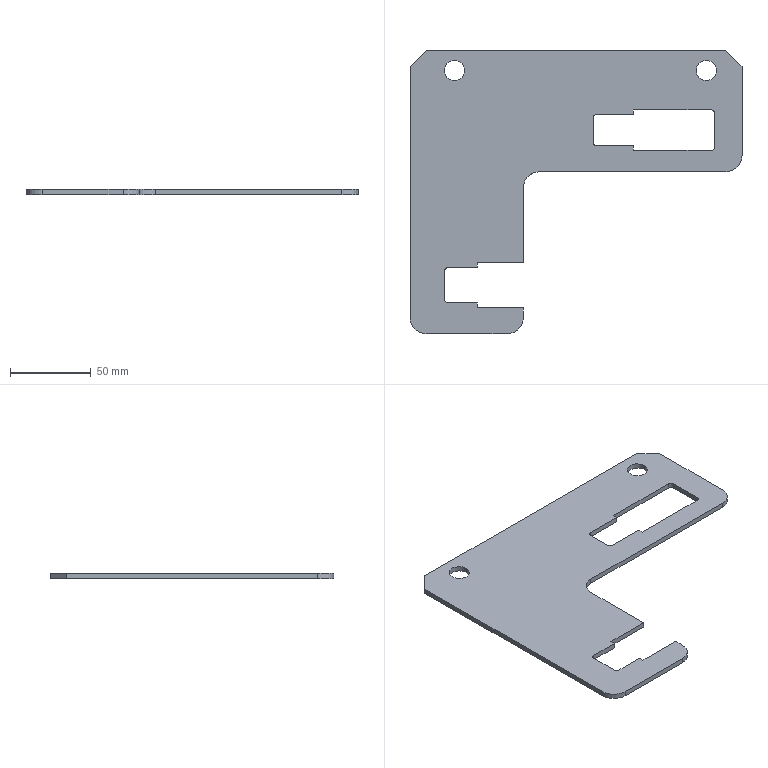Part | SolidWorks | features FlatPattern 1, SMBaseFlange 1, SheetMetal 1 | 1 solid | 40 faces | box 205 x 175 x 3.2 mm | volume 60892 mm3 | plane 26 | cylinder 14 | commonest cylinder face diameters 4 x6 12.5 x4 20 x4
STEP:
#1=CARTESIAN_POINT('',(21.25,-130.495,3.2));
#2=VERTEX_POINT('',#1);
#3=CARTESIAN_POINT('',(33.75,-130.495,3.2));
#4=VERTEX_POINT('',#3);
#5=CARTESIAN_POINT('',(27.5,-130.495,3.2));
#6=DIRECTION('',(0.,0.,1.));
#7=DIRECTION('',(1.,0.,0.));
#8=AXIS2_PLACEMENT_3D('',#5,#6,#7);
#9=CIRCLE('',#8,6.25);
#10=EDGE_CURVE('',#2,#4,#9,.T.);
#11=ORIENTED_EDGE('',*,*,#10,.T.);
#12=CARTESIAN_POINT('',(33.75,-130.495,0.));
#13=VERTEX_POINT('',#12);
#14=CARTESIAN_POINT('',(33.75,-130.495,3.2));
#15=DIRECTION('',(0.,0.,-1.));
#16=VECTOR('',#15,1000.);
#17=LINE('',#14,#16);
#18=EDGE_CURVE('',#4,#13,#17,.T.);
#19=ORIENTED_EDGE('',*,*,#18,.T.);
#20=CARTESIAN_POINT('',(21.25,-130.495,0.));
#21=VERTEX_POINT('',#20);
#22=CARTESIAN_POINT('',(27.5,-130.495,0.));
#23=DIRECTION('',(0.,0.,1.));
#24=DIRECTION('',(1.,0.,0.));
#25=AXIS2_PLACEMENT_3D('',#22,#23,#24);
#26=CIRCLE('',#25,6.25);
#27=EDGE_CURVE('',#21,#13,#26,.T.);
#28=ORIENTED_EDGE('',*,*,#27,.F.);
#29=CARTESIAN_POINT('',(21.25,-130.495,3.2));
#30=DIRECTION('',(0.,0.,-1.));
#31=VECTOR('',#30,1000.);
#32=LINE('',#29,#31);
#33=EDGE_CURVE('',#2,#21,#32,.T.);
#34=ORIENTED_EDGE('',*,*,#33,.F.);
#35=EDGE_LOOP('',(#11,#19,#28,#34));
#36=FACE_OUTER_BOUND('',#35,.T.);
#37=CARTESIAN_POINT('',(27.5,-130.495,3.2));
#38=DIRECTION('',(0.,0.,-1.));
#39=DIRECTION('',(-1.,0.,0.));
#40=AXIS2_PLACEMENT_3D('',#37,#38,#39);
#41=CYLINDRICAL_SURFACE('',#40,6.25);
#42=ADVANCED_FACE('',(#36),#41,.F.);
#43=CARTESIAN_POINT('',(176.75,-130.495,3.2));
#44=VERTEX_POINT('',#43);
#45=CARTESIAN_POINT('',(189.25,-130.495,3.2));
#46=VERTEX_POINT('',#45);
#47=CARTESIAN_POINT('',(183.,-130.495,3.2));
#48=DIRECTION('',(0.,0.,1.));
#49=DIRECTION('',(1.,0.,0.));
#50=AXIS2_PLACEMENT_3D('',#47,#48,#49);
#51=CIRCLE('',#50,6.25);
#52=EDGE_CURVE('',#44,#46,#51,.T.);
#53=ORIENTED_EDGE('',*,*,#52,.T.);
#54=CARTESIAN_POINT('',(189.25,-130.495,0.));
#55=VERTEX_POINT('',#54);
#56=CARTESIAN_POINT('',(189.25,-130.495,3.2));
#57=DIRECTION('',(0.,0.,-1.));
#58=VECTOR('',#57,1000.);
#59=LINE('',#56,#58);
#60=EDGE_CURVE('',#46,#55,#59,.T.);
#61=ORIENTED_EDGE('',*,*,#60,.T.);
#62=CARTESIAN_POINT('',(176.75,-130.495,0.));
#63=VERTEX_POINT('',#62);
#64=CARTESIAN_POINT('',(183.,-130.495,0.));
#65=DIRECTION('',(0.,0.,1.));
#66=DIRECTION('',(1.,0.,0.));
#67=AXIS2_PLACEMENT_3D('',#64,#65,#66);
#68=CIRCLE('',#67,6.25);
#69=EDGE_CURVE('',#63,#55,#68,.T.);
#70=ORIENTED_EDGE('',*,*,#69,.F.);
#71=CARTESIAN_POINT('',(176.75,-130.495,3.2));
#72=DIRECTION('',(0.,0.,-1.));
#73=VECTOR('',#72,1000.);
#74=LINE('',#71,#73);
#75=EDGE_CURVE('',#44,#63,#74,.T.);
#76=ORIENTED_EDGE('',*,*,#75,.F.);
#77=EDGE_LOOP('',(#53,#61,#70,#76));
#78=FACE_OUTER_BOUND('',#77,.T.);
#79=CARTESIAN_POINT('',(183.,-130.495,3.2));
#80=DIRECTION('',(0.,0.,-1.));
#81=DIRECTION('',(-1.,0.,0.));
#82=AXIS2_PLACEMENT_3D('',#79,#80,#81);
#83=CYLINDRICAL_SURFACE('',#82,6.25);
#84=ADVANCED_FACE('',(#78),#83,.F.);
#85=ORIENTED_EDGE('',*,*,#52,.F.);
#86=CARTESIAN_POINT('',(183.,-130.495,3.2));
#87=DIRECTION('',(0.,0.,1.));
#88=DIRECTION('',(1.,0.,0.));
#89=AXIS2_PLACEMENT_3D('',#86,#87,#88);
#90=CIRCLE('',#89,6.25);
#91=EDGE_CURVE('',#46,#44,#90,.T.);
#92=ORIENTED_EDGE('',*,*,#91,.F.);
#93=EDGE_LOOP('',(#85,#92));
#94=FACE_BOUND('',#93,.T.);
#95=CARTESIAN_POINT('',(205.,-182.995,3.2));
#96=VERTEX_POINT('',#95);
#97=CARTESIAN_POINT('',(205.,-127.995,3.2));
#98=VERTEX_POINT('',#97);
#99=CARTESIAN_POINT('',(205.,-154.795,3.2));
#100=DIRECTION('',(0.,1.,0.));
#101=VECTOR('',#100,1000.);
#102=LINE('',#99,#101);
#103=EDGE_CURVE('',#96,#98,#102,.T.);
#104=ORIENTED_EDGE('',*,*,#103,.T.);
#105=CARTESIAN_POINT('',(195.,-117.995,3.2));
#106=VERTEX_POINT('',#105);
#107=CARTESIAN_POINT('',(205.,-127.995,3.2));
#108=DIRECTION('',(-0.7071,0.7071,0.));
#109=VECTOR('',#108,1000.);
#110=LINE('',#107,#109);
#111=EDGE_CURVE('',#98,#106,#110,.T.);
#112=ORIENTED_EDGE('',*,*,#111,.T.);
#113=CARTESIAN_POINT('',(10.,-117.995,3.2));
#114=VERTEX_POINT('',#113);
#115=CARTESIAN_POINT('',(195.,-117.995,3.2));
#116=DIRECTION('',(-1.,0.,0.));
#117=VECTOR('',#116,1000.);
#118=LINE('',#115,#117);
#119=EDGE_CURVE('',#106,#114,#118,.T.);
#120=ORIENTED_EDGE('',*,*,#119,.T.);
#121=CARTESIAN_POINT('',(0.,-127.995,3.2));
#122=VERTEX_POINT('',#121);
#123=CARTESIAN_POINT('',(10.,-117.995,3.2));
#124=DIRECTION('',(-0.7071,-0.7071,0.));
#125=VECTOR('',#124,1000.);
#126=LINE('',#123,#125);
#127=EDGE_CURVE('',#114,#122,#126,.T.);
#128=ORIENTED_EDGE('',*,*,#127,.T.);
#129=CARTESIAN_POINT('',(0.,-282.995,3.2));
#130=VERTEX_POINT('',#129);
#131=CARTESIAN_POINT('',(0.,-127.995,3.2));
#132=DIRECTION('',(0.,-1.,0.));
#133=VECTOR('',#132,1000.);
#134=LINE('',#131,#133);
#135=EDGE_CURVE('',#122,#130,#134,.T.);
#136=ORIENTED_EDGE('',*,*,#135,.T.);
#137=CARTESIAN_POINT('',(10.,-292.995,3.2));
#138=VERTEX_POINT('',#137);
#139=CARTESIAN_POINT('',(10.,-282.995,3.2));
#140=DIRECTION('',(0.,0.,1.));
#141=DIRECTION('',(1.,0.,0.));
#142=AXIS2_PLACEMENT_3D('',#139,#140,#141);
#143=CIRCLE('',#142,10.);
#144=EDGE_CURVE('',#130,#138,#143,.T.);
#145=ORIENTED_EDGE('',*,*,#144,.T.);
#146=CARTESIAN_POINT('',(60.,-292.995,3.2));
#147=VERTEX_POINT('',#146);
#148=CARTESIAN_POINT('',(10.,-292.995,3.2));
#149=DIRECTION('',(1.,0.,0.));
#150=VECTOR('',#149,1000.);
#151=LINE('',#148,#150);
#152=EDGE_CURVE('',#138,#147,#151,.T.);
#153=ORIENTED_EDGE('',*,*,#152,.T.);
#154=CARTESIAN_POINT('',(70.,-282.995,3.2));
#155=VERTEX_POINT('',#154);
#156=CARTESIAN_POINT('',(60.,-282.995,3.2));
#157=DIRECTION('',(0.,0.,1.));
#158=DIRECTION('',(-1.,0.,0.));
#159=AXIS2_PLACEMENT_3D('',#156,#157,#158);
#160=CIRCLE('',#159,10.);
#161=EDGE_CURVE('',#147,#155,#160,.T.);
#162=ORIENTED_EDGE('',*,*,#161,.T.);
#163=CARTESIAN_POINT('',(70.,-276.995,3.2));
#164=VERTEX_POINT('',#163);
#165=CARTESIAN_POINT('',(70.,-282.995,3.2));
#166=DIRECTION('',(0.,1.,0.));
#167=VECTOR('',#166,1000.);
#168=LINE('',#165,#167);
#169=EDGE_CURVE('',#155,#164,#168,.T.);
#170=ORIENTED_EDGE('',*,*,#169,.T.);
#171=CARTESIAN_POINT('',(41.5,-276.995,3.2));
#172=VERTEX_POINT('',#171);
#173=CARTESIAN_POINT('',(41.5,-276.995,3.2));
#174=DIRECTION('',(-1.,0.,0.));
#175=VECTOR('',#174,1000.);
#176=LINE('',#173,#175);
#177=EDGE_CURVE('',#164,#172,#176,.T.);
#178=ORIENTED_EDGE('',*,*,#177,.T.);
#179=CARTESIAN_POINT('',(41.5,-273.995,3.2));
#180=VERTEX_POINT('',#179);
#181=CARTESIAN_POINT('',(41.5,-273.995,3.2));
#182=DIRECTION('',(0.,1.,0.));
#183=VECTOR('',#182,1000.);
#184=LINE('',#181,#183);
#185=EDGE_CURVE('',#172,#180,#184,.T.);
#186=ORIENTED_EDGE('',*,*,#185,.T.);
#187=CARTESIAN_POINT('',(23.5,-273.995,3.2));
#188=VERTEX_POINT('',#187);
#189=CARTESIAN_POINT('',(23.5,-273.995,3.2));
#190=DIRECTION('',(-1.,0.,0.));
#191=VECTOR('',#190,1000.);
#192=LINE('',#189,#191);
#193=EDGE_CURVE('',#180,#188,#192,.T.);
#194=ORIENTED_EDGE('',*,*,#193,.T.);
#195=CARTESIAN_POINT('',(21.5,-271.995,3.2));
#196=VERTEX_POINT('',#195);
#197=CARTESIAN_POINT('',(23.5,-271.995,3.2));
#198=DIRECTION('',(0.,0.,-1.));
#199=DIRECTION('',(1.,0.,0.));
#200=AXIS2_PLACEMENT_3D('',#197,#198,#199);
#201=CIRCLE('',#200,2.);
#202=EDGE_CURVE('',#188,#196,#201,.T.);
#203=ORIENTED_EDGE('',*,*,#202,.T.);
#204=CARTESIAN_POINT('',(21.5,-253.995,3.2));
#205=VERTEX_POINT('',#204);
#206=CARTESIAN_POINT('',(21.5,-253.995,3.2));
#207=DIRECTION('',(0.,1.,0.));
#208=VECTOR('',#207,1000.);
#209=LINE('',#206,#208);
#210=EDGE_CURVE('',#196,#205,#209,.T.);
#211=ORIENTED_EDGE('',*,*,#210,.T.);
#212=CARTESIAN_POINT('',(23.5,-251.995,3.2));
#213=VERTEX_POINT('',#212);
#214=CARTESIAN_POINT('',(23.5,-253.995,3.2));
#215=DIRECTION('',(0.,0.,-1.));
#216=DIRECTION('',(1.,0.,0.));
#217=AXIS2_PLACEMENT_3D('',#214,#215,#216);
#218=CIRCLE('',#217,2.);
#219=EDGE_CURVE('',#205,#213,#218,.T.);
#220=ORIENTED_EDGE('',*,*,#219,.T.);
#221=CARTESIAN_POINT('',(41.5,-251.995,3.2));
#222=VERTEX_POINT('',#221);
#223=CARTESIAN_POINT('',(41.5,-251.995,3.2));
#224=DIRECTION('',(1.,0.,0.));
#225=VECTOR('',#224,1000.);
#226=LINE('',#223,#225);
#227=EDGE_CURVE('',#213,#222,#226,.T.);
#228=ORIENTED_EDGE('',*,*,#227,.T.);
#229=CARTESIAN_POINT('',(41.5,-248.995,3.2));
#230=VERTEX_POINT('',#229);
#231=CARTESIAN_POINT('',(41.5,-248.995,3.2));
#232=DIRECTION('',(0.,1.,0.));
#233=VECTOR('',#232,1000.);
#234=LINE('',#231,#233);
#235=EDGE_CURVE('',#222,#230,#234,.T.);
#236=ORIENTED_EDGE('',*,*,#235,.T.);
#237=CARTESIAN_POINT('',(70.,-248.995,3.2));
#238=VERTEX_POINT('',#237);
#239=CARTESIAN_POINT('',(70.,-248.995,3.2));
#240=DIRECTION('',(1.,0.,0.));
#241=VECTOR('',#240,1000.);
#242=LINE('',#239,#241);
#243=EDGE_CURVE('',#230,#238,#242,.T.);
#244=ORIENTED_EDGE('',*,*,#243,.T.);
#245=CARTESIAN_POINT('',(70.,-202.995,3.2));
#246=VERTEX_POINT('',#245);
#247=CARTESIAN_POINT('',(70.,-248.995,3.2));
#248=DIRECTION('',(0.,1.,0.));
#249=VECTOR('',#248,1000.);
#250=LINE('',#247,#249);
#251=EDGE_CURVE('',#238,#246,#250,.T.);
#252=ORIENTED_EDGE('',*,*,#251,.T.);
#253=CARTESIAN_POINT('',(80.,-192.995,3.2));
#254=VERTEX_POINT('',#253);
#255=CARTESIAN_POINT('',(80.,-202.995,3.2));
#256=DIRECTION('',(0.,0.,-1.));
#257=DIRECTION('',(-1.,0.,0.));
#258=AXIS2_PLACEMENT_3D('',#255,#256,#257);
#259=CIRCLE('',#258,10.);
#260=EDGE_CURVE('',#246,#254,#259,.T.);
#261=ORIENTED_EDGE('',*,*,#260,.T.);
#262=CARTESIAN_POINT('',(195.,-192.995,3.2));
#263=VERTEX_POINT('',#262);
#264=CARTESIAN_POINT('',(80.,-192.995,3.2));
#265=DIRECTION('',(1.,0.,0.));
#266=VECTOR('',#265,1000.);
#267=LINE('',#264,#266);
#268=EDGE_CURVE('',#254,#263,#267,.T.);
#269=ORIENTED_EDGE('',*,*,#268,.T.);
#270=CARTESIAN_POINT('',(195.,-182.995,3.2));
#271=DIRECTION('',(0.,0.,1.));
#272=DIRECTION('',(1.,0.,0.));
#273=AXIS2_PLACEMENT_3D('',#270,#271,#272);
#274=CIRCLE('',#273,10.);
#275=EDGE_CURVE('',#263,#96,#274,.T.);
#276=ORIENTED_EDGE('',*,*,#275,.T.);
#277=EDGE_LOOP('',(#104,#112,#120,#128,#136,#145,#153,#162,#170,#178,#186,#194,#203,#211,#220,#228,#236,#244,#252,#261,#269,#276));
#278=FACE_OUTER_BOUND('',#277,.T.);
#279=ORIENTED_EDGE('',*,*,#10,.F.);
#280=CARTESIAN_POINT('',(27.5,-130.495,3.2));
#281=DIRECTION('',(0.,0.,1.));
#282=DIRECTION('',(1.,0.,0.));
#283=AXIS2_PLACEMENT_3D('',#280,#281,#282);
#284=CIRCLE('',#283,6.25);
#285=EDGE_CURVE('',#4,#2,#284,.T.);
#286=ORIENTED_EDGE('',*,*,#285,.F.);
#287=EDGE_LOOP('',(#279,#286));
#288=FACE_BOUND('',#287,.T.);
#289=CARTESIAN_POINT('',(138.,-157.795,3.2));
#290=VERTEX_POINT('',#289);
#291=CARTESIAN_POINT('',(115.,-157.795,3.2));
#292=VERTEX_POINT('',#291);
#293=CARTESIAN_POINT('',(138.,-157.795,3.2));
#294=DIRECTION('',(-1.,0.,0.));
#295=VECTOR('',#294,1000.);
#296=LINE('',#293,#295);
#297=EDGE_CURVE('',#290,#292,#296,.T.);
#298=ORIENTED_EDGE('',*,*,#297,.F.);
#299=CARTESIAN_POINT('',(138.,-154.795,3.2));
#300=VERTEX_POINT('',#299);
#301=CARTESIAN_POINT('',(138.,-154.795,3.2));
#302=DIRECTION('',(0.,-1.,0.));
#303=VECTOR('',#302,1000.);
#304=LINE('',#301,#303);
#305=EDGE_CURVE('',#300,#290,#304,.T.);
#306=ORIENTED_EDGE('',*,*,#305,.F.);
#307=CARTESIAN_POINT('',(186.,-154.795,3.2));
#308=VERTEX_POINT('',#307);
#309=CARTESIAN_POINT('',(186.,-154.795,3.2));
#310=DIRECTION('',(-1.,0.,0.));
#311=VECTOR('',#310,1000.);
#312=LINE('',#309,#311);
#313=EDGE_CURVE('',#308,#300,#312,.T.);
#314=ORIENTED_EDGE('',*,*,#313,.F.);
#315=CARTESIAN_POINT('',(188.,-156.795,3.2));
#316=VERTEX_POINT('',#315);
#317=CARTESIAN_POINT('',(186.,-156.795,3.2));
#318=DIRECTION('',(0.,0.,1.));
#319=DIRECTION('',(1.,0.,0.));
#320=AXIS2_PLACEMENT_3D('',#317,#318,#319);
#321=CIRCLE('',#320,2.);
#322=EDGE_CURVE('',#316,#308,#321,.T.);
#323=ORIENTED_EDGE('',*,*,#322,.F.);
#324=CARTESIAN_POINT('',(188.,-177.795,3.2));
#325=VERTEX_POINT('',#324);
#326=CARTESIAN_POINT('',(188.,-156.795,3.2));
#327=DIRECTION('',(0.,1.,0.));
#328=VECTOR('',#327,1000.);
#329=LINE('',#326,#328);
#330=EDGE_CURVE('',#325,#316,#329,.T.);
#331=ORIENTED_EDGE('',*,*,#330,.F.);
#332=CARTESIAN_POINT('',(186.,-179.795,3.2));
#333=VERTEX_POINT('',#332);
#334=CARTESIAN_POINT('',(186.,-177.795,3.2));
#335=DIRECTION('',(0.,0.,1.));
#336=DIRECTION('',(-1.,0.,0.));
#337=AXIS2_PLACEMENT_3D('',#334,#335,#336);
#338=CIRCLE('',#337,2.);
#339=EDGE_CURVE('',#333,#325,#338,.T.);
#340=ORIENTED_EDGE('',*,*,#339,.F.);
#341=CARTESIAN_POINT('',(138.,-179.795,3.2));
#342=VERTEX_POINT('',#341);
#343=CARTESIAN_POINT('',(138.,-179.795,3.2));
#344=DIRECTION('',(1.,0.,0.));
#345=VECTOR('',#344,1000.);
#346=LINE('',#343,#345);
#347=EDGE_CURVE('',#342,#333,#346,.T.);
#348=ORIENTED_EDGE('',*,*,#347,.F.);
#349=CARTESIAN_POINT('',(138.,-176.795,3.2));
#350=VERTEX_POINT('',#349);
#351=CARTESIAN_POINT('',(138.,-176.795,3.2));
#352=DIRECTION('',(0.,-1.,0.));
#353=VECTOR('',#352,1000.);
#354=LINE('',#351,#353);
#355=EDGE_CURVE('',#350,#342,#354,.T.);
#356=ORIENTED_EDGE('',*,*,#355,.F.);
#357=CARTESIAN_POINT('',(115.,-176.795,3.2));
#358=VERTEX_POINT('',#357);
#359=CARTESIAN_POINT('',(115.,-176.795,3.2));
#360=DIRECTION('',(1.,0.,0.));
#361=VECTOR('',#360,1000.);
#362=LINE('',#359,#361);
#363=EDGE_CURVE('',#358,#350,#362,.T.);
#364=ORIENTED_EDGE('',*,*,#363,.F.);
#365=CARTESIAN_POINT('',(113.,-174.795,3.2));
#366=VERTEX_POINT('',#365);
#367=CARTESIAN_POINT('',(115.,-174.795,3.2));
#368=DIRECTION('',(0.,0.,1.));
#369=DIRECTION('',(1.,0.,0.));
#370=AXIS2_PLACEMENT_3D('',#367,#368,#369);
#371=CIRCLE('',#370,2.);
#372=EDGE_CURVE('',#366,#358,#371,.T.);
#373=ORIENTED_EDGE('',*,*,#372,.F.);
#374=CARTESIAN_POINT('',(113.,-159.795,3.2));
#375=VERTEX_POINT('',#374);
#376=CARTESIAN_POINT('',(113.,-159.795,3.2));
#377=DIRECTION('',(0.,-1.,0.));
#378=VECTOR('',#377,1000.);
#379=LINE('',#376,#378);
#380=EDGE_CURVE('',#375,#366,#379,.T.);
#381=ORIENTED_EDGE('',*,*,#380,.F.);
#382=CARTESIAN_POINT('',(115.,-159.795,3.2));
#383=DIRECTION('',(0.,0.,1.));
#384=DIRECTION('',(1.,0.,0.));
#385=AXIS2_PLACEMENT_3D('',#382,#383,#384);
#386=CIRCLE('',#385,2.);
#387=EDGE_CURVE('',#292,#375,#386,.T.);
#388=ORIENTED_EDGE('',*,*,#387,.F.);
#389=EDGE_LOOP('',(#298,#306,#314,#323,#331,#340,#348,#356,#364,#373,#381,#388));
#390=FACE_BOUND('',#389,.T.);
#391=CARTESIAN_POINT('',(10.,-282.995,3.2));
#392=DIRECTION('',(0.,0.,1.));
#393=DIRECTION('',(1.,0.,0.));
#394=AXIS2_PLACEMENT_3D('',#391,#392,#393);
#395=PLANE('',#394);
#396=ADVANCED_FACE('',(#94,#278,#288,#390),#395,.T.);
#397=ORIENTED_EDGE('',*,*,#27,.T.);
#398=CARTESIAN_POINT('',(27.5,-130.495,0.));
#399=DIRECTION('',(0.,0.,1.));
#400=DIRECTION('',(1.,0.,0.));
#401=AXIS2_PLACEMENT_3D('',#398,#399,#400);
#402=CIRCLE('',#401,6.25);
#403=EDGE_CURVE('',#13,#21,#402,.T.);
#404=ORIENTED_EDGE('',*,*,#403,.T.);
#405=EDGE_LOOP('',(#397,#404));
#406=FACE_BOUND('',#405,.T.);
#407=ORIENTED_EDGE('',*,*,#69,.T.);
#408=CARTESIAN_POINT('',(183.,-130.495,0.));
#409=DIRECTION('',(0.,0.,1.));
#410=DIRECTION('',(1.,0.,0.));
#411=AXIS2_PLACEMENT_3D('',#408,#409,#410);
#412=CIRCLE('',#411,6.25);
#413=EDGE_CURVE('',#55,#63,#412,.T.);
#414=ORIENTED_EDGE('',*,*,#413,.T.);
#415=EDGE_LOOP('',(#407,#414));
#416=FACE_BOUND('',#415,.T.);
#417=CARTESIAN_POINT('',(205.,-127.995,0.));
#418=VERTEX_POINT('',#417);
#419=CARTESIAN_POINT('',(195.,-117.995,0.));
#420=VERTEX_POINT('',#419);
#421=CARTESIAN_POINT('',(205.,-127.995,0.));
#422=DIRECTION('',(-0.7071,0.7071,0.));
#423=VECTOR('',#422,1000.);
#424=LINE('',#421,#423);
#425=EDGE_CURVE('',#418,#420,#424,.T.);
#426=ORIENTED_EDGE('',*,*,#425,.F.);
#427=CARTESIAN_POINT('',(205.,-182.995,0.));
#428=VERTEX_POINT('',#427);
#429=CARTESIAN_POINT('',(205.,-182.995,0.));
#430=DIRECTION('',(0.,1.,0.));
#431=VECTOR('',#430,1000.);
#432=LINE('',#429,#431);
#433=EDGE_CURVE('',#428,#418,#432,.T.);
#434=ORIENTED_EDGE('',*,*,#433,.F.);
#435=CARTESIAN_POINT('',(195.,-192.995,0.));
#436=VERTEX_POINT('',#435);
#437=CARTESIAN_POINT('',(195.,-182.995,0.));
#438=DIRECTION('',(0.,0.,1.));
#439=DIRECTION('',(1.,0.,0.));
#440=AXIS2_PLACEMENT_3D('',#437,#438,#439);
#441=CIRCLE('',#440,10.);
#442=EDGE_CURVE('',#436,#428,#441,.T.);
#443=ORIENTED_EDGE('',*,*,#442,.F.);
#444=CARTESIAN_POINT('',(80.,-192.995,0.));
#445=VERTEX_POINT('',#444);
#446=CARTESIAN_POINT('',(80.,-192.995,0.));
#447=DIRECTION('',(1.,0.,0.));
#448=VECTOR('',#447,1000.);
#449=LINE('',#446,#448);
#450=EDGE_CURVE('',#445,#436,#449,.T.);
#451=ORIENTED_EDGE('',*,*,#450,.F.);
#452=CARTESIAN_POINT('',(70.,-202.995,0.));
#453=VERTEX_POINT('',#452);
#454=CARTESIAN_POINT('',(80.,-202.995,0.));
#455=DIRECTION('',(0.,0.,-1.));
#456=DIRECTION('',(-1.,0.,0.));
#457=AXIS2_PLACEMENT_3D('',#454,#455,#456);
#458=CIRCLE('',#457,10.);
#459=EDGE_CURVE('',#453,#445,#458,.T.);
#460=ORIENTED_EDGE('',*,*,#459,.F.);
#461=CARTESIAN_POINT('',(70.,-248.995,0.));
#462=VERTEX_POINT('',#461);
#463=CARTESIAN_POINT('',(70.,-248.995,0.));
#464=DIRECTION('',(0.,1.,0.));
#465=VECTOR('',#464,1000.);
#466=LINE('',#463,#465);
#467=EDGE_CURVE('',#462,#453,#466,.T.);
#468=ORIENTED_EDGE('',*,*,#467,.F.);
#469=CARTESIAN_POINT('',(41.5,-248.995,0.));
#470=VERTEX_POINT('',#469);
#471=CARTESIAN_POINT('',(70.,-248.995,0.));
#472=DIRECTION('',(1.,0.,0.));
#473=VECTOR('',#472,1000.);
#474=LINE('',#471,#473);
#475=EDGE_CURVE('',#470,#462,#474,.T.);
#476=ORIENTED_EDGE('',*,*,#475,.F.);
#477=CARTESIAN_POINT('',(41.5,-251.995,0.));
#478=VERTEX_POINT('',#477);
#479=CARTESIAN_POINT('',(41.5,-248.995,0.));
#480=DIRECTION('',(0.,1.,0.));
#481=VECTOR('',#480,1000.);
#482=LINE('',#479,#481);
#483=EDGE_CURVE('',#478,#470,#482,.T.);
#484=ORIENTED_EDGE('',*,*,#483,.F.);
#485=CARTESIAN_POINT('',(23.5,-251.995,0.));
#486=VERTEX_POINT('',#485);
#487=CARTESIAN_POINT('',(41.5,-251.995,0.));
#488=DIRECTION('',(1.,0.,0.));
#489=VECTOR('',#488,1000.);
#490=LINE('',#487,#489);
#491=EDGE_CURVE('',#486,#478,#490,.T.);
#492=ORIENTED_EDGE('',*,*,#491,.F.);
#493=CARTESIAN_POINT('',(21.5,-253.995,0.));
#494=VERTEX_POINT('',#493);
#495=CARTESIAN_POINT('',(23.5,-253.995,0.));
#496=DIRECTION('',(0.,0.,-1.));
#497=DIRECTION('',(1.,0.,0.));
#498=AXIS2_PLACEMENT_3D('',#495,#496,#497);
#499=CIRCLE('',#498,2.);
#500=EDGE_CURVE('',#494,#486,#499,.T.);
#501=ORIENTED_EDGE('',*,*,#500,.F.);
#502=CARTESIAN_POINT('',(21.5,-271.995,0.));
#503=VERTEX_POINT('',#502);
#504=CARTESIAN_POINT('',(21.5,-253.995,0.));
#505=DIRECTION('',(0.,1.,0.));
#506=VECTOR('',#505,1000.);
#507=LINE('',#504,#506);
#508=EDGE_CURVE('',#503,#494,#507,.T.);
#509=ORIENTED_EDGE('',*,*,#508,.F.);
#510=CARTESIAN_POINT('',(23.5,-273.995,0.));
#511=VERTEX_POINT('',#510);
#512=CARTESIAN_POINT('',(23.5,-271.995,0.));
#513=DIRECTION('',(0.,0.,-1.));
#514=DIRECTION('',(1.,0.,0.));
#515=AXIS2_PLACEMENT_3D('',#512,#513,#514);
#516=CIRCLE('',#515,2.);
#517=EDGE_CURVE('',#511,#503,#516,.T.);
#518=ORIENTED_EDGE('',*,*,#517,.F.);
#519=CARTESIAN_POINT('',(41.5,-273.995,0.));
#520=VERTEX_POINT('',#519);
#521=CARTESIAN_POINT('',(23.5,-273.995,0.));
#522=DIRECTION('',(-1.,0.,0.));
#523=VECTOR('',#522,1000.);
#524=LINE('',#521,#523);
#525=EDGE_CURVE('',#520,#511,#524,.T.);
#526=ORIENTED_EDGE('',*,*,#525,.F.);
#527=CARTESIAN_POINT('',(41.5,-276.995,0.));
#528=VERTEX_POINT('',#527);
#529=CARTESIAN_POINT('',(41.5,-273.995,0.));
#530=DIRECTION('',(0.,1.,0.));
#531=VECTOR('',#530,1000.);
#532=LINE('',#529,#531);
#533=EDGE_CURVE('',#528,#520,#532,.T.);
#534=ORIENTED_EDGE('',*,*,#533,.F.);
#535=CARTESIAN_POINT('',(70.,-276.995,0.));
#536=VERTEX_POINT('',#535);
#537=CARTESIAN_POINT('',(41.5,-276.995,0.));
#538=DIRECTION('',(-1.,0.,0.));
#539=VECTOR('',#538,1000.);
#540=LINE('',#537,#539);
#541=EDGE_CURVE('',#536,#528,#540,.T.);
#542=ORIENTED_EDGE('',*,*,#541,.F.);
#543=CARTESIAN_POINT('',(70.,-282.995,0.));
#544=VERTEX_POINT('',#543);
#545=CARTESIAN_POINT('',(70.,-282.995,0.));
#546=DIRECTION('',(0.,1.,0.));
#547=VECTOR('',#546,1000.);
#548=LINE('',#545,#547);
#549=EDGE_CURVE('',#544,#536,#548,.T.);
#550=ORIENTED_EDGE('',*,*,#549,.F.);
#551=CARTESIAN_POINT('',(60.,-292.995,0.));
#552=VERTEX_POINT('',#551);
#553=CARTESIAN_POINT('',(60.,-282.995,0.));
#554=DIRECTION('',(0.,0.,1.));
#555=DIRECTION('',(-1.,0.,0.));
#556=AXIS2_PLACEMENT_3D('',#553,#554,#555);
#557=CIRCLE('',#556,10.);
#558=EDGE_CURVE('',#552,#544,#557,.T.);
#559=ORIENTED_EDGE('',*,*,#558,.F.);
#560=CARTESIAN_POINT('',(10.,-292.995,0.));
#561=VERTEX_POINT('',#560);
#562=CARTESIAN_POINT('',(10.,-292.995,0.));
#563=DIRECTION('',(1.,0.,0.));
#564=VECTOR('',#563,1000.);
#565=LINE('',#562,#564);
#566=EDGE_CURVE('',#561,#552,#565,.T.);
#567=ORIENTED_EDGE('',*,*,#566,.F.);
#568=CARTESIAN_POINT('',(0.,-282.995,0.));
#569=VERTEX_POINT('',#568);
#570=CARTESIAN_POINT('',(10.,-282.995,0.));
#571=DIRECTION('',(0.,0.,1.));
#572=DIRECTION('',(1.,0.,0.));
#573=AXIS2_PLACEMENT_3D('',#570,#571,#572);
#574=CIRCLE('',#573,10.);
#575=EDGE_CURVE('',#569,#561,#574,.T.);
#576=ORIENTED_EDGE('',*,*,#575,.F.);
#577=CARTESIAN_POINT('',(0.,-127.995,0.));
#578=VERTEX_POINT('',#577);
#579=CARTESIAN_POINT('',(0.,-127.995,0.));
#580=DIRECTION('',(0.,-1.,0.));
#581=VECTOR('',#580,1000.);
#582=LINE('',#579,#581);
#583=EDGE_CURVE('',#578,#569,#582,.T.);
#584=ORIENTED_EDGE('',*,*,#583,.F.);
#585=CARTESIAN_POINT('',(10.,-117.995,0.));
#586=VERTEX_POINT('',#585);
#587=CARTESIAN_POINT('',(10.,-117.995,0.));
#588=DIRECTION('',(-0.7071,-0.7071,0.));
#589=VECTOR('',#588,1000.);
#590=LINE('',#587,#589);
#591=EDGE_CURVE('',#586,#578,#590,.T.);
#592=ORIENTED_EDGE('',*,*,#591,.F.);
#593=CARTESIAN_POINT('',(195.,-117.995,0.));
#594=DIRECTION('',(-1.,0.,0.));
#595=VECTOR('',#594,1000.);
#596=LINE('',#593,#595);
#597=EDGE_CURVE('',#420,#586,#596,.T.);
#598=ORIENTED_EDGE('',*,*,#597,.F.);
#599=EDGE_LOOP('',(#426,#434,#443,#451,#460,#468,#476,#484,#492,#501,#509,#518,#526,#534,#542,#550,#559,#567,#576,#584,#592,#598));
#600=FACE_OUTER_BOUND('',#599,.T.);
#601=CARTESIAN_POINT('',(138.,-154.795,0.));
#602=VERTEX_POINT('',#601);
#603=CARTESIAN_POINT('',(138.,-157.795,0.));
#604=VERTEX_POINT('',#603);
#605=CARTESIAN_POINT('',(138.,-154.795,0.));
#606=DIRECTION('',(0.,-1.,0.));
#607=VECTOR('',#606,1000.);
#608=LINE('',#605,#607);
#609=EDGE_CURVE('',#602,#604,#608,.T.);
#610=ORIENTED_EDGE('',*,*,#609,.T.);
#611=CARTESIAN_POINT('',(115.,-157.795,0.));
#612=VERTEX_POINT('',#611);
#613=CARTESIAN_POINT('',(138.,-157.795,0.));
#614=DIRECTION('',(-1.,0.,0.));
#615=VECTOR('',#614,1000.);
#616=LINE('',#613,#615);
#617=EDGE_CURVE('',#604,#612,#616,.T.);
#618=ORIENTED_EDGE('',*,*,#617,.T.);
#619=CARTESIAN_POINT('',(113.,-159.795,0.));
#620=VERTEX_POINT('',#619);
#621=CARTESIAN_POINT('',(115.,-159.795,0.));
#622=DIRECTION('',(0.,0.,1.));
#623=DIRECTION('',(1.,0.,0.));
#624=AXIS2_PLACEMENT_3D('',#621,#622,#623);
#625=CIRCLE('',#624,2.);
#626=EDGE_CURVE('',#612,#620,#625,.T.);
#627=ORIENTED_EDGE('',*,*,#626,.T.);
#628=CARTESIAN_POINT('',(113.,-174.795,0.));
#629=VERTEX_POINT('',#628);
#630=CARTESIAN_POINT('',(113.,-159.795,0.));
#631=DIRECTION('',(0.,-1.,0.));
#632=VECTOR('',#631,1000.);
#633=LINE('',#630,#632);
#634=EDGE_CURVE('',#620,#629,#633,.T.);
#635=ORIENTED_EDGE('',*,*,#634,.T.);
#636=CARTESIAN_POINT('',(115.,-176.795,0.));
#637=VERTEX_POINT('',#636);
#638=CARTESIAN_POINT('',(115.,-174.795,0.));
#639=DIRECTION('',(0.,0.,1.));
#640=DIRECTION('',(1.,0.,0.));
#641=AXIS2_PLACEMENT_3D('',#638,#639,#640);
#642=CIRCLE('',#641,2.);
#643=EDGE_CURVE('',#629,#637,#642,.T.);
#644=ORIENTED_EDGE('',*,*,#643,.T.);
#645=CARTESIAN_POINT('',(138.,-176.795,0.));
#646=VERTEX_POINT('',#645);
#647=CARTESIAN_POINT('',(115.,-176.795,0.));
#648=DIRECTION('',(1.,0.,0.));
#649=VECTOR('',#648,1000.);
#650=LINE('',#647,#649);
#651=EDGE_CURVE('',#637,#646,#650,.T.);
#652=ORIENTED_EDGE('',*,*,#651,.T.);
#653=CARTESIAN_POINT('',(138.,-179.795,0.));
#654=VERTEX_POINT('',#653);
#655=CARTESIAN_POINT('',(138.,-176.795,0.));
#656=DIRECTION('',(0.,-1.,0.));
#657=VECTOR('',#656,1000.);
#658=LINE('',#655,#657);
#659=EDGE_CURVE('',#646,#654,#658,.T.);
#660=ORIENTED_EDGE('',*,*,#659,.T.);
#661=CARTESIAN_POINT('',(186.,-179.795,0.));
#662=VERTEX_POINT('',#661);
#663=CARTESIAN_POINT('',(138.,-179.795,0.));
#664=DIRECTION('',(1.,0.,0.));
#665=VECTOR('',#664,1000.);
#666=LINE('',#663,#665);
#667=EDGE_CURVE('',#654,#662,#666,.T.);
#668=ORIENTED_EDGE('',*,*,#667,.T.);
#669=CARTESIAN_POINT('',(188.,-177.795,0.));
#670=VERTEX_POINT('',#669);
#671=CARTESIAN_POINT('',(186.,-177.795,0.));
#672=DIRECTION('',(0.,0.,1.));
#673=DIRECTION('',(-1.,0.,0.));
#674=AXIS2_PLACEMENT_3D('',#671,#672,#673);
#675=CIRCLE('',#674,2.);
#676=EDGE_CURVE('',#662,#670,#675,.T.);
#677=ORIENTED_EDGE('',*,*,#676,.T.);
#678=CARTESIAN_POINT('',(188.,-156.795,0.));
#679=VERTEX_POINT('',#678);
#680=CARTESIAN_POINT('',(188.,-156.795,0.));
#681=DIRECTION('',(0.,1.,0.));
#682=VECTOR('',#681,1000.);
#683=LINE('',#680,#682);
#684=EDGE_CURVE('',#670,#679,#683,.T.);
#685=ORIENTED_EDGE('',*,*,#684,.T.);
#686=CARTESIAN_POINT('',(186.,-154.795,0.));
#687=VERTEX_POINT('',#686);
#688=CARTESIAN_POINT('',(186.,-156.795,0.));
#689=DIRECTION('',(0.,0.,1.));
#690=DIRECTION('',(1.,0.,0.));
#691=AXIS2_PLACEMENT_3D('',#688,#689,#690);
#692=CIRCLE('',#691,2.);
#693=EDGE_CURVE('',#679,#687,#692,.T.);
#694=ORIENTED_EDGE('',*,*,#693,.T.);
#695=CARTESIAN_POINT('',(186.,-154.795,0.));
#696=DIRECTION('',(-1.,0.,0.));
#697=VECTOR('',#696,1000.);
#698=LINE('',#695,#697);
#699=EDGE_CURVE('',#687,#602,#698,.T.);
#700=ORIENTED_EDGE('',*,*,#699,.T.);
#701=EDGE_LOOP('',(#610,#618,#627,#635,#644,#652,#660,#668,#677,#685,#694,#700));
#702=FACE_BOUND('',#701,.T.);
#703=CARTESIAN_POINT('',(10.,-282.995,0.));
#704=DIRECTION('',(0.,0.,1.));
#705=DIRECTION('',(1.,0.,0.));
#706=AXIS2_PLACEMENT_3D('',#703,#704,#705);
#707=PLANE('',#706);
#708=ADVANCED_FACE('',(#406,#416,#600,#702),#707,.F.);
#709=ORIENTED_EDGE('',*,*,#425,.T.);
#710=CARTESIAN_POINT('',(195.,-117.995,3.2));
#711=DIRECTION('',(0.,0.,-1.));
#712=VECTOR('',#711,1000.);
#713=LINE('',#710,#712);
#714=EDGE_CURVE('',#106,#420,#713,.T.);
#715=ORIENTED_EDGE('',*,*,#714,.F.);
#716=ORIENTED_EDGE('',*,*,#111,.F.);
#717=CARTESIAN_POINT('',(205.,-127.995,3.2));
#718=DIRECTION('',(0.,0.,-1.));
#719=VECTOR('',#718,1000.);
#720=LINE('',#717,#719);
#721=EDGE_CURVE('',#98,#418,#720,.T.);
#722=ORIENTED_EDGE('',*,*,#721,.T.);
#723=EDGE_LOOP('',(#709,#715,#716,#722));
#724=FACE_OUTER_BOUND('',#723,.T.);
#725=CARTESIAN_POINT('',(205.,-127.995,3.2));
#726=DIRECTION('',(-0.7071,-0.7071,0.));
#727=DIRECTION('',(0.7071,-0.7071,0.));
#728=AXIS2_PLACEMENT_3D('',#725,#726,#727);
#729=PLANE('',#728);
#730=ADVANCED_FACE('',(#724),#729,.F.);
#731=ORIENTED_EDGE('',*,*,#597,.T.);
#732=CARTESIAN_POINT('',(10.,-117.995,3.2));
#733=DIRECTION('',(0.,0.,-1.));
#734=VECTOR('',#733,1000.);
#735=LINE('',#732,#734);
#736=EDGE_CURVE('',#114,#586,#735,.T.);
#737=ORIENTED_EDGE('',*,*,#736,.F.);
#738=ORIENTED_EDGE('',*,*,#119,.F.);
#739=ORIENTED_EDGE('',*,*,#714,.T.);
#740=EDGE_LOOP('',(#731,#737,#738,#739));
#741=FACE_OUTER_BOUND('',#740,.T.);
#742=CARTESIAN_POINT('',(195.,-117.995,3.2));
#743=DIRECTION('',(0.,-1.,0.));
#744=DIRECTION('',(0.,0.,-1.));
#745=AXIS2_PLACEMENT_3D('',#742,#743,#744);
#746=PLANE('',#745);
#747=ADVANCED_FACE('',(#741),#746,.F.);
#748=ORIENTED_EDGE('',*,*,#591,.T.);
#749=CARTESIAN_POINT('',(0.,-127.995,3.2));
#750=DIRECTION('',(0.,0.,-1.));
#751=VECTOR('',#750,1000.);
#752=LINE('',#749,#751);
#753=EDGE_CURVE('',#122,#578,#752,.T.);
#754=ORIENTED_EDGE('',*,*,#753,.F.);
#755=ORIENTED_EDGE('',*,*,#127,.F.);
#756=ORIENTED_EDGE('',*,*,#736,.T.);
#757=EDGE_LOOP('',(#748,#754,#755,#756));
#758=FACE_OUTER_BOUND('',#757,.T.);
#759=CARTESIAN_POINT('',(10.,-117.995,3.2));
#760=DIRECTION('',(0.7071,-0.7071,0.));
#761=DIRECTION('',(0.7071,0.7071,0.));
#762=AXIS2_PLACEMENT_3D('',#759,#760,#761);
#763=PLANE('',#762);
#764=ADVANCED_FACE('',(#758),#763,.F.);
#765=ORIENTED_EDGE('',*,*,#583,.T.);
#766=CARTESIAN_POINT('',(0.,-282.995,3.2));
#767=DIRECTION('',(0.,0.,-1.));
#768=VECTOR('',#767,1000.);
#769=LINE('',#766,#768);
#770=EDGE_CURVE('',#130,#569,#769,.T.);
#771=ORIENTED_EDGE('',*,*,#770,.F.);
#772=ORIENTED_EDGE('',*,*,#135,.F.);
#773=ORIENTED_EDGE('',*,*,#753,.T.);
#774=EDGE_LOOP('',(#765,#771,#772,#773));
#775=FACE_OUTER_BOUND('',#774,.T.);
#776=CARTESIAN_POINT('',(0.,-127.995,3.2));
#777=DIRECTION('',(1.,0.,0.));
#778=DIRECTION('',(0.,1.,0.));
#779=AXIS2_PLACEMENT_3D('',#776,#777,#778);
#780=PLANE('',#779);
#781=ADVANCED_FACE('',(#775),#780,.F.);
#782=ORIENTED_EDGE('',*,*,#575,.T.);
#783=CARTESIAN_POINT('',(10.,-292.995,3.2));
#784=DIRECTION('',(0.,0.,-1.));
#785=VECTOR('',#784,1000.);
#786=LINE('',#783,#785);
#787=EDGE_CURVE('',#138,#561,#786,.T.);
#788=ORIENTED_EDGE('',*,*,#787,.F.);
#789=ORIENTED_EDGE('',*,*,#144,.F.);
#790=ORIENTED_EDGE('',*,*,#770,.T.);
#791=EDGE_LOOP('',(#782,#788,#789,#790));
#792=FACE_OUTER_BOUND('',#791,.T.);
#793=CARTESIAN_POINT('',(10.,-282.995,3.2));
#794=DIRECTION('',(0.,0.,-1.));
#795=DIRECTION('',(-1.,0.,0.));
#796=AXIS2_PLACEMENT_3D('',#793,#794,#795);
#797=CYLINDRICAL_SURFACE('',#796,10.);
#798=ADVANCED_FACE('',(#792),#797,.T.);
#799=ORIENTED_EDGE('',*,*,#566,.T.);
#800=CARTESIAN_POINT('',(60.,-292.995,3.2));
#801=DIRECTION('',(0.,0.,-1.));
#802=VECTOR('',#801,1000.);
#803=LINE('',#800,#802);
#804=EDGE_CURVE('',#147,#552,#803,.T.);
#805=ORIENTED_EDGE('',*,*,#804,.F.);
#806=ORIENTED_EDGE('',*,*,#152,.F.);
#807=ORIENTED_EDGE('',*,*,#787,.T.);
#808=EDGE_LOOP('',(#799,#805,#806,#807));
#809=FACE_OUTER_BOUND('',#808,.T.);
#810=CARTESIAN_POINT('',(10.,-292.995,3.2));
#811=DIRECTION('',(0.,1.,0.));
#812=DIRECTION('',(0.,0.,1.));
#813=AXIS2_PLACEMENT_3D('',#810,#811,#812);
#814=PLANE('',#813);
#815=ADVANCED_FACE('',(#809),#814,.F.);
#816=ORIENTED_EDGE('',*,*,#558,.T.);
#817=CARTESIAN_POINT('',(70.,-282.995,3.2));
#818=DIRECTION('',(0.,0.,-1.));
#819=VECTOR('',#818,1000.);
#820=LINE('',#817,#819);
#821=EDGE_CURVE('',#155,#544,#820,.T.);
#822=ORIENTED_EDGE('',*,*,#821,.F.);
#823=ORIENTED_EDGE('',*,*,#161,.F.);
#824=ORIENTED_EDGE('',*,*,#804,.T.);
#825=EDGE_LOOP('',(#816,#822,#823,#824));
#826=FACE_OUTER_BOUND('',#825,.T.);
#827=CARTESIAN_POINT('',(60.,-282.995,3.2));
#828=DIRECTION('',(0.,0.,-1.));
#829=DIRECTION('',(-1.,0.,0.));
#830=AXIS2_PLACEMENT_3D('',#827,#828,#829);
#831=CYLINDRICAL_SURFACE('',#830,10.);
#832=ADVANCED_FACE('',(#826),#831,.T.);
#833=ORIENTED_EDGE('',*,*,#549,.T.);
#834=CARTESIAN_POINT('',(70.,-276.995,3.2));
#835=DIRECTION('',(0.,0.,-1.));
#836=VECTOR('',#835,1000.);
#837=LINE('',#834,#836);
#838=EDGE_CURVE('',#164,#536,#837,.T.);
#839=ORIENTED_EDGE('',*,*,#838,.F.);
#840=ORIENTED_EDGE('',*,*,#169,.F.);
#841=ORIENTED_EDGE('',*,*,#821,.T.);
#842=EDGE_LOOP('',(#833,#839,#840,#841));
#843=FACE_OUTER_BOUND('',#842,.T.);
#844=CARTESIAN_POINT('',(70.,-282.995,3.2));
#845=DIRECTION('',(-1.,0.,0.));
#846=DIRECTION('',(0.,0.,1.));
#847=AXIS2_PLACEMENT_3D('',#844,#845,#846);
#848=PLANE('',#847);
#849=ADVANCED_FACE('',(#843),#848,.F.);
#850=ORIENTED_EDGE('',*,*,#541,.T.);
#851=CARTESIAN_POINT('',(41.5,-276.995,3.2));
#852=DIRECTION('',(0.,0.,-1.));
#853=VECTOR('',#852,1000.);
#854=LINE('',#851,#853);
#855=EDGE_CURVE('',#172,#528,#854,.T.);
#856=ORIENTED_EDGE('',*,*,#855,.F.);
#857=ORIENTED_EDGE('',*,*,#177,.F.);
#858=ORIENTED_EDGE('',*,*,#838,.T.);
#859=EDGE_LOOP('',(#850,#856,#857,#858));
#860=FACE_OUTER_BOUND('',#859,.T.);
#861=CARTESIAN_POINT('',(41.5,-276.995,3.2));
#862=DIRECTION('',(0.,-1.,0.));
#863=DIRECTION('',(0.,0.,-1.));
#864=AXIS2_PLACEMENT_3D('',#861,#862,#863);
#865=PLANE('',#864);
#866=ADVANCED_FACE('',(#860),#865,.F.);
#867=ORIENTED_EDGE('',*,*,#533,.T.);
#868=CARTESIAN_POINT('',(41.5,-273.995,3.2));
#869=DIRECTION('',(0.,0.,-1.));
#870=VECTOR('',#869,1000.);
#871=LINE('',#868,#870);
#872=EDGE_CURVE('',#180,#520,#871,.T.);
#873=ORIENTED_EDGE('',*,*,#872,.F.);
#874=ORIENTED_EDGE('',*,*,#185,.F.);
#875=ORIENTED_EDGE('',*,*,#855,.T.);
#876=EDGE_LOOP('',(#867,#873,#874,#875));
#877=FACE_OUTER_BOUND('',#876,.T.);
#878=CARTESIAN_POINT('',(41.5,-273.995,3.2));
#879=DIRECTION('',(-1.,0.,0.));
#880=DIRECTION('',(0.,0.,1.));
#881=AXIS2_PLACEMENT_3D('',#878,#879,#880);
#882=PLANE('',#881);
#883=ADVANCED_FACE('',(#877),#882,.F.);
#884=ORIENTED_EDGE('',*,*,#525,.T.);
#885=CARTESIAN_POINT('',(23.5,-273.995,3.2));
#886=DIRECTION('',(0.,0.,-1.));
#887=VECTOR('',#886,1000.);
#888=LINE('',#885,#887);
#889=EDGE_CURVE('',#188,#511,#888,.T.);
#890=ORIENTED_EDGE('',*,*,#889,.F.);
#891=ORIENTED_EDGE('',*,*,#193,.F.);
#892=ORIENTED_EDGE('',*,*,#872,.T.);
#893=EDGE_LOOP('',(#884,#890,#891,#892));
#894=FACE_OUTER_BOUND('',#893,.T.);
#895=CARTESIAN_POINT('',(23.5,-273.995,3.2));
#896=DIRECTION('',(0.,-1.,0.));
#897=DIRECTION('',(0.,0.,-1.));
#898=AXIS2_PLACEMENT_3D('',#895,#896,#897);
#899=PLANE('',#898);
#900=ADVANCED_FACE('',(#894),#899,.F.);
#901=ORIENTED_EDGE('',*,*,#517,.T.);
#902=CARTESIAN_POINT('',(21.5,-271.995,3.2));
#903=DIRECTION('',(0.,0.,-1.));
#904=VECTOR('',#903,1000.);
#905=LINE('',#902,#904);
#906=EDGE_CURVE('',#196,#503,#905,.T.);
#907=ORIENTED_EDGE('',*,*,#906,.F.);
#908=ORIENTED_EDGE('',*,*,#202,.F.);
#909=ORIENTED_EDGE('',*,*,#889,.T.);
#910=EDGE_LOOP('',(#901,#907,#908,#909));
#911=FACE_OUTER_BOUND('',#910,.T.);
#912=CARTESIAN_POINT('',(23.5,-271.995,3.2));
#913=DIRECTION('',(0.,0.,-1.));
#914=DIRECTION('',(-1.,0.,0.));
#915=AXIS2_PLACEMENT_3D('',#912,#913,#914);
#916=CYLINDRICAL_SURFACE('',#915,2.);
#917=ADVANCED_FACE('',(#911),#916,.F.);
#918=ORIENTED_EDGE('',*,*,#508,.T.);
#919=CARTESIAN_POINT('',(21.5,-253.995,3.2));
#920=DIRECTION('',(0.,0.,-1.));
#921=VECTOR('',#920,1000.);
#922=LINE('',#919,#921);
#923=EDGE_CURVE('',#205,#494,#922,.T.);
#924=ORIENTED_EDGE('',*,*,#923,.F.);
#925=ORIENTED_EDGE('',*,*,#210,.F.);
#926=ORIENTED_EDGE('',*,*,#906,.T.);
#927=EDGE_LOOP('',(#918,#924,#925,#926));
#928=FACE_OUTER_BOUND('',#927,.T.);
#929=CARTESIAN_POINT('',(21.5,-253.995,3.2));
#930=DIRECTION('',(-1.,0.,0.));
#931=DIRECTION('',(0.,0.,1.));
#932=AXIS2_PLACEMENT_3D('',#929,#930,#931);
#933=PLANE('',#932);
#934=ADVANCED_FACE('',(#928),#933,.F.);
#935=ORIENTED_EDGE('',*,*,#500,.T.);
#936=CARTESIAN_POINT('',(23.5,-251.995,3.2));
#937=DIRECTION('',(0.,0.,-1.));
#938=VECTOR('',#937,1000.);
#939=LINE('',#936,#938);
#940=EDGE_CURVE('',#213,#486,#939,.T.);
#941=ORIENTED_EDGE('',*,*,#940,.F.);
#942=ORIENTED_EDGE('',*,*,#219,.F.);
#943=ORIENTED_EDGE('',*,*,#923,.T.);
#944=EDGE_LOOP('',(#935,#941,#942,#943));
#945=FACE_OUTER_BOUND('',#944,.T.);
#946=CARTESIAN_POINT('',(23.5,-253.995,3.2));
#947=DIRECTION('',(0.,0.,-1.));
#948=DIRECTION('',(-1.,0.,0.));
#949=AXIS2_PLACEMENT_3D('',#946,#947,#948);
#950=CYLINDRICAL_SURFACE('',#949,2.);
#951=ADVANCED_FACE('',(#945),#950,.F.);
#952=ORIENTED_EDGE('',*,*,#491,.T.);
#953=CARTESIAN_POINT('',(41.5,-251.995,3.2));
#954=DIRECTION('',(0.,0.,-1.));
#955=VECTOR('',#954,1000.);
#956=LINE('',#953,#955);
#957=EDGE_CURVE('',#222,#478,#956,.T.);
#958=ORIENTED_EDGE('',*,*,#957,.F.);
#959=ORIENTED_EDGE('',*,*,#227,.F.);
#960=ORIENTED_EDGE('',*,*,#940,.T.);
#961=EDGE_LOOP('',(#952,#958,#959,#960));
#962=FACE_OUTER_BOUND('',#961,.T.);
#963=CARTESIAN_POINT('',(41.5,-251.995,3.2));
#964=DIRECTION('',(0.,1.,0.));
#965=DIRECTION('',(0.,0.,1.));
#966=AXIS2_PLACEMENT_3D('',#963,#964,#965);
#967=PLANE('',#966);
#968=ADVANCED_FACE('',(#962),#967,.F.);
#969=ORIENTED_EDGE('',*,*,#483,.T.);
#970=CARTESIAN_POINT('',(41.5,-248.995,3.2));
#971=DIRECTION('',(0.,0.,-1.));
#972=VECTOR('',#971,1000.);
#973=LINE('',#970,#972);
#974=EDGE_CURVE('',#230,#470,#973,.T.);
#975=ORIENTED_EDGE('',*,*,#974,.F.);
#976=ORIENTED_EDGE('',*,*,#235,.F.);
#977=ORIENTED_EDGE('',*,*,#957,.T.);
#978=EDGE_LOOP('',(#969,#975,#976,#977));
#979=FACE_OUTER_BOUND('',#978,.T.);
#980=CARTESIAN_POINT('',(41.5,-248.995,3.2));
#981=DIRECTION('',(-1.,0.,0.));
#982=DIRECTION('',(0.,0.,1.));
#983=AXIS2_PLACEMENT_3D('',#980,#981,#982);
#984=PLANE('',#983);
#985=ADVANCED_FACE('',(#979),#984,.F.);
#986=ORIENTED_EDGE('',*,*,#475,.T.);
#987=CARTESIAN_POINT('',(70.,-248.995,3.2));
#988=DIRECTION('',(0.,0.,-1.));
#989=VECTOR('',#988,1000.);
#990=LINE('',#987,#989);
#991=EDGE_CURVE('',#238,#462,#990,.T.);
#992=ORIENTED_EDGE('',*,*,#991,.F.);
#993=ORIENTED_EDGE('',*,*,#243,.F.);
#994=ORIENTED_EDGE('',*,*,#974,.T.);
#995=EDGE_LOOP('',(#986,#992,#993,#994));
#996=FACE_OUTER_BOUND('',#995,.T.);
#997=CARTESIAN_POINT('',(70.,-248.995,3.2));
#998=DIRECTION('',(0.,1.,0.));
#999=DIRECTION('',(0.,0.,1.));
#1000=AXIS2_PLACEMENT_3D('',#997,#998,#999);
#1001=PLANE('',#1000);
#1002=ADVANCED_FACE('',(#996),#1001,.F.);
#1003=ORIENTED_EDGE('',*,*,#467,.T.);
#1004=CARTESIAN_POINT('',(70.,-202.995,3.2));
#1005=DIRECTION('',(0.,0.,-1.));
#1006=VECTOR('',#1005,1000.);
#1007=LINE('',#1004,#1006);
#1008=EDGE_CURVE('',#246,#453,#1007,.T.);
#1009=ORIENTED_EDGE('',*,*,#1008,.F.);
#1010=ORIENTED_EDGE('',*,*,#251,.F.);
#1011=ORIENTED_EDGE('',*,*,#991,.T.);
#1012=EDGE_LOOP('',(#1003,#1009,#1010,#1011));
#1013=FACE_OUTER_BOUND('',#1012,.T.);
#1014=CARTESIAN_POINT('',(70.,-248.995,3.2));
#1015=DIRECTION('',(-1.,0.,0.));
#1016=DIRECTION('',(0.,0.,1.));
#1017=AXIS2_PLACEMENT_3D('',#1014,#1015,#1016);
#1018=PLANE('',#1017);
#1019=ADVANCED_FACE('',(#1013),#1018,.F.);
#1020=ORIENTED_EDGE('',*,*,#459,.T.);
#1021=CARTESIAN_POINT('',(80.,-192.995,3.2));
#1022=DIRECTION('',(0.,0.,-1.));
#1023=VECTOR('',#1022,1000.);
#1024=LINE('',#1021,#1023);
#1025=EDGE_CURVE('',#254,#445,#1024,.T.);
#1026=ORIENTED_EDGE('',*,*,#1025,.F.);
#1027=ORIENTED_EDGE('',*,*,#260,.F.);
#1028=ORIENTED_EDGE('',*,*,#1008,.T.);
#1029=EDGE_LOOP('',(#1020,#1026,#1027,#1028));
#1030=FACE_OUTER_BOUND('',#1029,.T.);
#1031=CARTESIAN_POINT('',(80.,-202.995,3.2));
#1032=DIRECTION('',(0.,0.,-1.));
#1033=DIRECTION('',(-1.,0.,0.));
#1034=AXIS2_PLACEMENT_3D('',#1031,#1032,#1033);
#1035=CYLINDRICAL_SURFACE('',#1034,10.);
#1036=ADVANCED_FACE('',(#1030),#1035,.F.);
#1037=ORIENTED_EDGE('',*,*,#450,.T.);
#1038=CARTESIAN_POINT('',(195.,-192.995,3.2));
#1039=DIRECTION('',(0.,0.,-1.));
#1040=VECTOR('',#1039,1000.);
#1041=LINE('',#1038,#1040);
#1042=EDGE_CURVE('',#263,#436,#1041,.T.);
#1043=ORIENTED_EDGE('',*,*,#1042,.F.);
#1044=ORIENTED_EDGE('',*,*,#268,.F.);
#1045=ORIENTED_EDGE('',*,*,#1025,.T.);
#1046=EDGE_LOOP('',(#1037,#1043,#1044,#1045));
#1047=FACE_OUTER_BOUND('',#1046,.T.);
#1048=CARTESIAN_POINT('',(80.,-192.995,3.2));
#1049=DIRECTION('',(0.,1.,0.));
#1050=DIRECTION('',(-1.,0.,0.));
#1051=AXIS2_PLACEMENT_3D('',#1048,#1049,#1050);
#1052=PLANE('',#1051);
#1053=ADVANCED_FACE('',(#1047),#1052,.F.);
#1054=ORIENTED_EDGE('',*,*,#442,.T.);
#1055=CARTESIAN_POINT('',(205.,-182.995,3.2));
#1056=DIRECTION('',(0.,0.,-1.));
#1057=VECTOR('',#1056,1000.);
#1058=LINE('',#1055,#1057);
#1059=EDGE_CURVE('',#96,#428,#1058,.T.);
#1060=ORIENTED_EDGE('',*,*,#1059,.F.);
#1061=ORIENTED_EDGE('',*,*,#275,.F.);
#1062=ORIENTED_EDGE('',*,*,#1042,.T.);
#1063=EDGE_LOOP('',(#1054,#1060,#1061,#1062));
#1064=FACE_OUTER_BOUND('',#1063,.T.);
#1065=CARTESIAN_POINT('',(195.,-182.995,3.2));
#1066=DIRECTION('',(0.,0.,-1.));
#1067=DIRECTION('',(-1.,0.,0.));
#1068=AXIS2_PLACEMENT_3D('',#1065,#1066,#1067);
#1069=CYLINDRICAL_SURFACE('',#1068,10.);
#1070=ADVANCED_FACE('',(#1064),#1069,.T.);
#1071=ORIENTED_EDGE('',*,*,#433,.T.);
#1072=ORIENTED_EDGE('',*,*,#721,.F.);
#1073=ORIENTED_EDGE('',*,*,#103,.F.);
#1074=ORIENTED_EDGE('',*,*,#1059,.T.);
#1075=EDGE_LOOP('',(#1071,#1072,#1073,#1074));
#1076=FACE_OUTER_BOUND('',#1075,.T.);
#1077=CARTESIAN_POINT('',(205.,-182.995,3.2));
#1078=DIRECTION('',(-1.,0.,0.));
#1079=DIRECTION('',(0.,0.,1.));
#1080=AXIS2_PLACEMENT_3D('',#1077,#1078,#1079);
#1081=PLANE('',#1080);
#1082=ADVANCED_FACE('',(#1076),#1081,.F.);
#1083=ORIENTED_EDGE('',*,*,#60,.F.);
#1084=ORIENTED_EDGE('',*,*,#91,.T.);
#1085=ORIENTED_EDGE('',*,*,#75,.T.);
#1086=ORIENTED_EDGE('',*,*,#413,.F.);
#1087=EDGE_LOOP('',(#1083,#1084,#1085,#1086));
#1088=FACE_OUTER_BOUND('',#1087,.T.);
#1089=CARTESIAN_POINT('',(183.,-130.495,3.2));
#1090=DIRECTION('',(0.,0.,-1.));
#1091=DIRECTION('',(-1.,0.,0.));
#1092=AXIS2_PLACEMENT_3D('',#1089,#1090,#1091);
#1093=CYLINDRICAL_SURFACE('',#1092,6.25);
#1094=ADVANCED_FACE('',(#1088),#1093,.F.);
#1095=ORIENTED_EDGE('',*,*,#18,.F.);
#1096=ORIENTED_EDGE('',*,*,#285,.T.);
#1097=ORIENTED_EDGE('',*,*,#33,.T.);
#1098=ORIENTED_EDGE('',*,*,#403,.F.);
#1099=EDGE_LOOP('',(#1095,#1096,#1097,#1098));
#1100=FACE_OUTER_BOUND('',#1099,.T.);
#1101=CARTESIAN_POINT('',(27.5,-130.495,3.2));
#1102=DIRECTION('',(0.,0.,-1.));
#1103=DIRECTION('',(-1.,0.,0.));
#1104=AXIS2_PLACEMENT_3D('',#1101,#1102,#1103);
#1105=CYLINDRICAL_SURFACE('',#1104,6.25);
#1106=ADVANCED_FACE('',(#1100),#1105,.F.);
#1107=ORIENTED_EDGE('',*,*,#609,.F.);
#1108=CARTESIAN_POINT('',(138.,-154.795,3.2));
#1109=DIRECTION('',(0.,0.,-1.));
#1110=VECTOR('',#1109,1000.);
#1111=LINE('',#1108,#1110);
#1112=EDGE_CURVE('',#300,#602,#1111,.T.);
#1113=ORIENTED_EDGE('',*,*,#1112,.F.);
#1114=ORIENTED_EDGE('',*,*,#305,.T.);
#1115=CARTESIAN_POINT('',(138.,-157.795,3.2));
#1116=DIRECTION('',(0.,0.,-1.));
#1117=VECTOR('',#1116,1000.);
#1118=LINE('',#1115,#1117);
#1119=EDGE_CURVE('',#290,#604,#1118,.T.);
#1120=ORIENTED_EDGE('',*,*,#1119,.T.);
#1121=EDGE_LOOP('',(#1107,#1113,#1114,#1120));
#1122=FACE_OUTER_BOUND('',#1121,.T.);
#1123=CARTESIAN_POINT('',(138.,-154.795,3.2));
#1124=DIRECTION('',(1.,0.,0.));
#1125=DIRECTION('',(0.,0.,-1.));
#1126=AXIS2_PLACEMENT_3D('',#1123,#1124,#1125);
#1127=PLANE('',#1126);
#1128=ADVANCED_FACE('',(#1122),#1127,.T.);
#1129=ORIENTED_EDGE('',*,*,#617,.F.);
#1130=ORIENTED_EDGE('',*,*,#1119,.F.);
#1131=ORIENTED_EDGE('',*,*,#297,.T.);
#1132=CARTESIAN_POINT('',(115.,-157.795,3.2));
#1133=DIRECTION('',(0.,0.,-1.));
#1134=VECTOR('',#1133,1000.);
#1135=LINE('',#1132,#1134);
#1136=EDGE_CURVE('',#292,#612,#1135,.T.);
#1137=ORIENTED_EDGE('',*,*,#1136,.T.);
#1138=EDGE_LOOP('',(#1129,#1130,#1131,#1137));
#1139=FACE_OUTER_BOUND('',#1138,.T.);
#1140=CARTESIAN_POINT('',(138.,-157.795,3.2));
#1141=DIRECTION('',(0.,-1.,0.));
#1142=DIRECTION('',(0.,0.,-1.));
#1143=AXIS2_PLACEMENT_3D('',#1140,#1141,#1142);
#1144=PLANE('',#1143);
#1145=ADVANCED_FACE('',(#1139),#1144,.T.);
#1146=ORIENTED_EDGE('',*,*,#626,.F.);
#1147=ORIENTED_EDGE('',*,*,#1136,.F.);
#1148=ORIENTED_EDGE('',*,*,#387,.T.);
#1149=CARTESIAN_POINT('',(113.,-159.795,3.2));
#1150=DIRECTION('',(0.,0.,-1.));
#1151=VECTOR('',#1150,1000.);
#1152=LINE('',#1149,#1151);
#1153=EDGE_CURVE('',#375,#620,#1152,.T.);
#1154=ORIENTED_EDGE('',*,*,#1153,.T.);
#1155=EDGE_LOOP('',(#1146,#1147,#1148,#1154));
#1156=FACE_OUTER_BOUND('',#1155,.T.);
#1157=CARTESIAN_POINT('',(115.,-159.795,3.2));
#1158=DIRECTION('',(0.,0.,-1.));
#1159=DIRECTION('',(-1.,0.,0.));
#1160=AXIS2_PLACEMENT_3D('',#1157,#1158,#1159);
#1161=CYLINDRICAL_SURFACE('',#1160,2.);
#1162=ADVANCED_FACE('',(#1156),#1161,.F.);
#1163=ORIENTED_EDGE('',*,*,#634,.F.);
#1164=ORIENTED_EDGE('',*,*,#1153,.F.);
#1165=ORIENTED_EDGE('',*,*,#380,.T.);
#1166=CARTESIAN_POINT('',(113.,-174.795,3.2));
#1167=DIRECTION('',(0.,0.,-1.));
#1168=VECTOR('',#1167,1000.);
#1169=LINE('',#1166,#1168);
#1170=EDGE_CURVE('',#366,#629,#1169,.T.);
#1171=ORIENTED_EDGE('',*,*,#1170,.T.);
#1172=EDGE_LOOP('',(#1163,#1164,#1165,#1171));
#1173=FACE_OUTER_BOUND('',#1172,.T.);
#1174=CARTESIAN_POINT('',(113.,-159.795,3.2));
#1175=DIRECTION('',(1.,0.,0.));
#1176=DIRECTION('',(0.,0.,-1.));
#1177=AXIS2_PLACEMENT_3D('',#1174,#1175,#1176);
#1178=PLANE('',#1177);
#1179=ADVANCED_FACE('',(#1173),#1178,.T.);
#1180=ORIENTED_EDGE('',*,*,#643,.F.);
#1181=ORIENTED_EDGE('',*,*,#1170,.F.);
#1182=ORIENTED_EDGE('',*,*,#372,.T.);
#1183=CARTESIAN_POINT('',(115.,-176.795,3.2));
#1184=DIRECTION('',(0.,0.,-1.));
#1185=VECTOR('',#1184,1000.);
#1186=LINE('',#1183,#1185);
#1187=EDGE_CURVE('',#358,#637,#1186,.T.);
#1188=ORIENTED_EDGE('',*,*,#1187,.T.);
#1189=EDGE_LOOP('',(#1180,#1181,#1182,#1188));
#1190=FACE_OUTER_BOUND('',#1189,.T.);
#1191=CARTESIAN_POINT('',(115.,-174.795,3.2));
#1192=DIRECTION('',(0.,0.,-1.));
#1193=DIRECTION('',(-1.,0.,0.));
#1194=AXIS2_PLACEMENT_3D('',#1191,#1192,#1193);
#1195=CYLINDRICAL_SURFACE('',#1194,2.);
#1196=ADVANCED_FACE('',(#1190),#1195,.F.);
#1197=ORIENTED_EDGE('',*,*,#651,.F.);
#1198=ORIENTED_EDGE('',*,*,#1187,.F.);
#1199=ORIENTED_EDGE('',*,*,#363,.T.);
#1200=CARTESIAN_POINT('',(138.,-176.795,3.2));
#1201=DIRECTION('',(0.,0.,-1.));
#1202=VECTOR('',#1201,1000.);
#1203=LINE('',#1200,#1202);
#1204=EDGE_CURVE('',#350,#646,#1203,.T.);
#1205=ORIENTED_EDGE('',*,*,#1204,.T.);
#1206=EDGE_LOOP('',(#1197,#1198,#1199,#1205));
#1207=FACE_OUTER_BOUND('',#1206,.T.);
#1208=CARTESIAN_POINT('',(115.,-176.795,3.2));
#1209=DIRECTION('',(0.,1.,0.));
#1210=DIRECTION('',(0.,0.,1.));
#1211=AXIS2_PLACEMENT_3D('',#1208,#1209,#1210);
#1212=PLANE('',#1211);
#1213=ADVANCED_FACE('',(#1207),#1212,.T.);
#1214=ORIENTED_EDGE('',*,*,#659,.F.);
#1215=ORIENTED_EDGE('',*,*,#1204,.F.);
#1216=ORIENTED_EDGE('',*,*,#355,.T.);
#1217=CARTESIAN_POINT('',(138.,-179.795,3.2));
#1218=DIRECTION('',(0.,0.,-1.));
#1219=VECTOR('',#1218,1000.);
#1220=LINE('',#1217,#1219);
#1221=EDGE_CURVE('',#342,#654,#1220,.T.);
#1222=ORIENTED_EDGE('',*,*,#1221,.T.);
#1223=EDGE_LOOP('',(#1214,#1215,#1216,#1222));
#1224=FACE_OUTER_BOUND('',#1223,.T.);
#1225=CARTESIAN_POINT('',(138.,-176.795,3.2));
#1226=DIRECTION('',(1.,0.,0.));
#1227=DIRECTION('',(0.,0.,-1.));
#1228=AXIS2_PLACEMENT_3D('',#1225,#1226,#1227);
#1229=PLANE('',#1228);
#1230=ADVANCED_FACE('',(#1224),#1229,.T.);
#1231=ORIENTED_EDGE('',*,*,#667,.F.);
#1232=ORIENTED_EDGE('',*,*,#1221,.F.);
#1233=ORIENTED_EDGE('',*,*,#347,.T.);
#1234=CARTESIAN_POINT('',(186.,-179.795,3.2));
#1235=DIRECTION('',(0.,0.,-1.));
#1236=VECTOR('',#1235,1000.);
#1237=LINE('',#1234,#1236);
#1238=EDGE_CURVE('',#333,#662,#1237,.T.);
#1239=ORIENTED_EDGE('',*,*,#1238,.T.);
#1240=EDGE_LOOP('',(#1231,#1232,#1233,#1239));
#1241=FACE_OUTER_BOUND('',#1240,.T.);
#1242=CARTESIAN_POINT('',(138.,-179.795,3.2));
#1243=DIRECTION('',(0.,1.,0.));
#1244=DIRECTION('',(0.,0.,1.));
#1245=AXIS2_PLACEMENT_3D('',#1242,#1243,#1244);
#1246=PLANE('',#1245);
#1247=ADVANCED_FACE('',(#1241),#1246,.T.);
#1248=ORIENTED_EDGE('',*,*,#676,.F.);
#1249=ORIENTED_EDGE('',*,*,#1238,.F.);
#1250=ORIENTED_EDGE('',*,*,#339,.T.);
#1251=CARTESIAN_POINT('',(188.,-177.795,3.2));
#1252=DIRECTION('',(0.,0.,-1.));
#1253=VECTOR('',#1252,1000.);
#1254=LINE('',#1251,#1253);
#1255=EDGE_CURVE('',#325,#670,#1254,.T.);
#1256=ORIENTED_EDGE('',*,*,#1255,.T.);
#1257=EDGE_LOOP('',(#1248,#1249,#1250,#1256));
#1258=FACE_OUTER_BOUND('',#1257,.T.);
#1259=CARTESIAN_POINT('',(186.,-177.795,3.2));
#1260=DIRECTION('',(0.,0.,-1.));
#1261=DIRECTION('',(-1.,0.,0.));
#1262=AXIS2_PLACEMENT_3D('',#1259,#1260,#1261);
#1263=CYLINDRICAL_SURFACE('',#1262,2.);
#1264=ADVANCED_FACE('',(#1258),#1263,.F.);
#1265=ORIENTED_EDGE('',*,*,#684,.F.);
#1266=ORIENTED_EDGE('',*,*,#1255,.F.);
#1267=ORIENTED_EDGE('',*,*,#330,.T.);
#1268=CARTESIAN_POINT('',(188.,-156.795,3.2));
#1269=DIRECTION('',(0.,0.,-1.));
#1270=VECTOR('',#1269,1000.);
#1271=LINE('',#1268,#1270);
#1272=EDGE_CURVE('',#316,#679,#1271,.T.);
#1273=ORIENTED_EDGE('',*,*,#1272,.T.);
#1274=EDGE_LOOP('',(#1265,#1266,#1267,#1273));
#1275=FACE_OUTER_BOUND('',#1274,.T.);
#1276=CARTESIAN_POINT('',(188.,-156.795,3.2));
#1277=DIRECTION('',(-1.,0.,0.));
#1278=DIRECTION('',(0.,0.,1.));
#1279=AXIS2_PLACEMENT_3D('',#1276,#1277,#1278);
#1280=PLANE('',#1279);
#1281=ADVANCED_FACE('',(#1275),#1280,.T.);
#1282=ORIENTED_EDGE('',*,*,#693,.F.);
#1283=ORIENTED_EDGE('',*,*,#1272,.F.);
#1284=ORIENTED_EDGE('',*,*,#322,.T.);
#1285=CARTESIAN_POINT('',(186.,-154.795,3.2));
#1286=DIRECTION('',(0.,0.,-1.));
#1287=VECTOR('',#1286,1000.);
#1288=LINE('',#1285,#1287);
#1289=EDGE_CURVE('',#308,#687,#1288,.T.);
#1290=ORIENTED_EDGE('',*,*,#1289,.T.);
#1291=EDGE_LOOP('',(#1282,#1283,#1284,#1290));
#1292=FACE_OUTER_BOUND('',#1291,.T.);
#1293=CARTESIAN_POINT('',(186.,-156.795,3.2));
#1294=DIRECTION('',(0.,0.,-1.));
#1295=DIRECTION('',(-1.,0.,0.));
#1296=AXIS2_PLACEMENT_3D('',#1293,#1294,#1295);
#1297=CYLINDRICAL_SURFACE('',#1296,2.);
#1298=ADVANCED_FACE('',(#1292),#1297,.F.);
#1299=ORIENTED_EDGE('',*,*,#699,.F.);
#1300=ORIENTED_EDGE('',*,*,#1289,.F.);
#1301=ORIENTED_EDGE('',*,*,#313,.T.);
#1302=ORIENTED_EDGE('',*,*,#1112,.T.);
#1303=EDGE_LOOP('',(#1299,#1300,#1301,#1302));
#1304=FACE_OUTER_BOUND('',#1303,.T.);
#1305=CARTESIAN_POINT('',(186.,-154.795,3.2));
#1306=DIRECTION('',(0.,-1.,0.));
#1307=DIRECTION('',(0.,0.,-1.));
#1308=AXIS2_PLACEMENT_3D('',#1305,#1306,#1307);
#1309=PLANE('',#1308);
#1310=ADVANCED_FACE('',(#1304),#1309,.T.);
#1311=CLOSED_SHELL('',(#42,#84,#396,#708,#730,#747,#764,#781,#798,#815,#832,#849,#866,#883,#900,#917,#934,#951,#968,#985,#1002,#1019,#1036,#1053,#1070,#1082,#1094,#1106,#1128,#1145,#1162,#1179,#1196,#1213,#1230,#1247,#1264,#1281,#1298,#1310));
#1312=MANIFOLD_SOLID_BREP('',#1311);
#1313=CARTESIAN_POINT('',(0.,0.,0.));
#1314=DIRECTION('',(0.,0.,1.));
#1315=DIRECTION('',(1.,0.,0.));
#1316=AXIS2_PLACEMENT_3D('',#1313,#1314,#1315);
#1317=(LENGTH_UNIT()NAMED_UNIT(*)SI_UNIT(.MILLI.,.METRE.));
#1318=UNCERTAINTY_MEASURE_WITH_UNIT(LENGTH_MEASURE(0.00001),#1317,'','');
#1319=(NAMED_UNIT(*)PLANE_ANGLE_UNIT()SI_UNIT($,.RADIAN.));
#1320=(NAMED_UNIT(*)SI_UNIT($,.STERADIAN.)SOLID_ANGLE_UNIT());
#1321=(GEOMETRIC_REPRESENTATION_CONTEXT(3)GLOBAL_UNCERTAINTY_ASSIGNED_CONTEXT((#1318))GLOBAL_UNIT_ASSIGNED_CONTEXT((#1317,#1319,#1320))REPRESENTATION_CONTEXT('',''));
#1322=ADVANCED_BREP_SHAPE_REPRESENTATION('',(#1312,#1316),#1321);